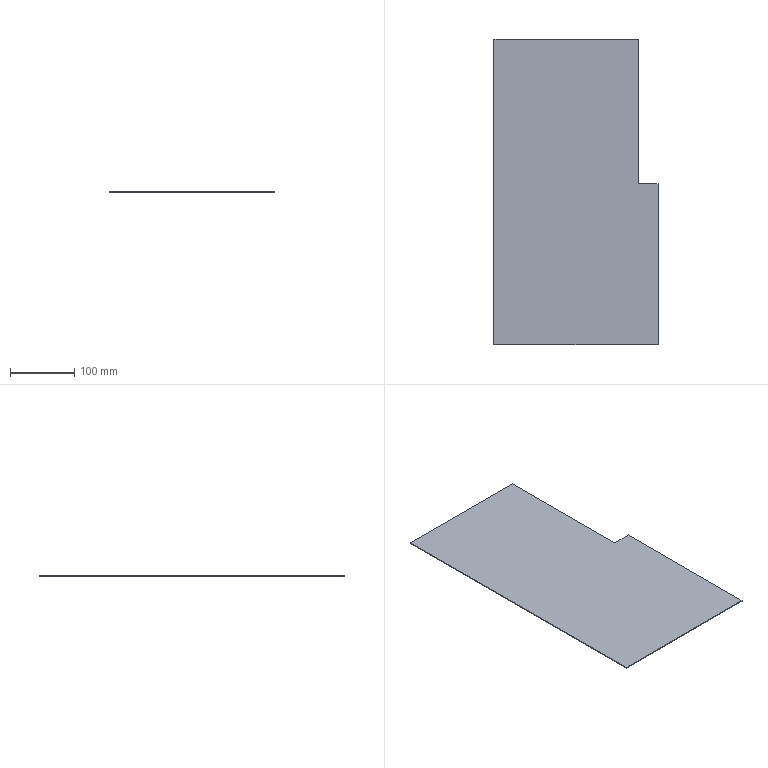Part | 1 solid | 8 faces | box 255 x 475 x 1.2 mm | volume 137250 mm3 | plane 8
STEP:
#1=CARTESIAN_POINT('',(97.5,237.5,0.));
#2=VERTEX_POINT('',#1);
#3=CARTESIAN_POINT('',(97.5,12.5,0.));
#4=VERTEX_POINT('',#3);
#5=CARTESIAN_POINT('',(97.5,0.,0.));
#6=DIRECTION('',(0.,-1.,0.));
#7=VECTOR('',#6,1000.);
#8=LINE('',#5,#7);
#9=EDGE_CURVE('',#2,#4,#8,.T.);
#10=ORIENTED_EDGE('',*,*,#9,.F.);
#11=CARTESIAN_POINT('',(97.5,237.5,1.2));
#12=VERTEX_POINT('',#11);
#13=CARTESIAN_POINT('',(97.5,237.5,1.2));
#14=DIRECTION('',(0.,0.,-1.));
#15=VECTOR('',#14,1000.);
#16=LINE('',#13,#15);
#17=EDGE_CURVE('',#12,#2,#16,.T.);
#18=ORIENTED_EDGE('',*,*,#17,.F.);
#19=CARTESIAN_POINT('',(97.5,12.5,1.2));
#20=VERTEX_POINT('',#19);
#21=CARTESIAN_POINT('',(97.5,0.,1.2));
#22=DIRECTION('',(0.,-1.,0.));
#23=VECTOR('',#22,1000.);
#24=LINE('',#21,#23);
#25=EDGE_CURVE('',#12,#20,#24,.T.);
#26=ORIENTED_EDGE('',*,*,#25,.T.);
#27=CARTESIAN_POINT('',(97.5,12.5,1.2));
#28=DIRECTION('',(0.,0.,-1.));
#29=VECTOR('',#28,1000.);
#30=LINE('',#27,#29);
#31=EDGE_CURVE('',#20,#4,#30,.T.);
#32=ORIENTED_EDGE('',*,*,#31,.T.);
#33=EDGE_LOOP('',(#10,#18,#26,#32));
#34=FACE_OUTER_BOUND('',#33,.T.);
#35=CARTESIAN_POINT('',(97.5,0.,1.2));
#36=DIRECTION('',(1.,0.,0.));
#37=DIRECTION('',(0.,1.,0.));
#38=AXIS2_PLACEMENT_3D('',#35,#36,#37);
#39=PLANE('',#38);
#40=ADVANCED_FACE('',(#34),#39,.T.);
#41=CARTESIAN_POINT('',(-127.5,237.5,0.));
#42=VERTEX_POINT('',#41);
#43=CARTESIAN_POINT('',(0.,237.5,0.));
#44=DIRECTION('',(1.,0.,0.));
#45=VECTOR('',#44,1000.);
#46=LINE('',#43,#45);
#47=EDGE_CURVE('',#42,#2,#46,.T.);
#48=ORIENTED_EDGE('',*,*,#47,.F.);
#49=CARTESIAN_POINT('',(-127.5,237.5,1.2));
#50=VERTEX_POINT('',#49);
#51=CARTESIAN_POINT('',(-127.5,237.5,1.2));
#52=DIRECTION('',(0.,0.,-1.));
#53=VECTOR('',#52,1000.);
#54=LINE('',#51,#53);
#55=EDGE_CURVE('',#50,#42,#54,.T.);
#56=ORIENTED_EDGE('',*,*,#55,.F.);
#57=CARTESIAN_POINT('',(0.,237.5,1.2));
#58=DIRECTION('',(1.,0.,0.));
#59=VECTOR('',#58,1000.);
#60=LINE('',#57,#59);
#61=EDGE_CURVE('',#50,#12,#60,.T.);
#62=ORIENTED_EDGE('',*,*,#61,.T.);
#63=ORIENTED_EDGE('',*,*,#17,.T.);
#64=EDGE_LOOP('',(#48,#56,#62,#63));
#65=FACE_OUTER_BOUND('',#64,.T.);
#66=CARTESIAN_POINT('',(0.,237.5,1.2));
#67=DIRECTION('',(0.,1.,0.));
#68=DIRECTION('',(0.,0.,1.));
#69=AXIS2_PLACEMENT_3D('',#66,#67,#68);
#70=PLANE('',#69);
#71=ADVANCED_FACE('',(#65),#70,.T.);
#72=CARTESIAN_POINT('',(-127.5,-237.5,0.));
#73=VERTEX_POINT('',#72);
#74=CARTESIAN_POINT('',(-127.5,0.,0.));
#75=DIRECTION('',(0.,-1.,0.));
#76=VECTOR('',#75,1000.);
#77=LINE('',#74,#76);
#78=EDGE_CURVE('',#42,#73,#77,.T.);
#79=ORIENTED_EDGE('',*,*,#78,.T.);
#80=CARTESIAN_POINT('',(-127.5,-237.5,1.2));
#81=VERTEX_POINT('',#80);
#82=CARTESIAN_POINT('',(-127.5,-237.5,1.2));
#83=DIRECTION('',(0.,0.,-1.));
#84=VECTOR('',#83,1000.);
#85=LINE('',#82,#84);
#86=EDGE_CURVE('',#81,#73,#85,.T.);
#87=ORIENTED_EDGE('',*,*,#86,.F.);
#88=CARTESIAN_POINT('',(-127.5,0.,1.2));
#89=DIRECTION('',(0.,-1.,0.));
#90=VECTOR('',#89,1000.);
#91=LINE('',#88,#90);
#92=EDGE_CURVE('',#50,#81,#91,.T.);
#93=ORIENTED_EDGE('',*,*,#92,.F.);
#94=ORIENTED_EDGE('',*,*,#55,.T.);
#95=EDGE_LOOP('',(#79,#87,#93,#94));
#96=FACE_OUTER_BOUND('',#95,.T.);
#97=CARTESIAN_POINT('',(-127.5,0.,1.2));
#98=DIRECTION('',(1.,0.,0.));
#99=DIRECTION('',(0.,1.,0.));
#100=AXIS2_PLACEMENT_3D('',#97,#98,#99);
#101=PLANE('',#100);
#102=ADVANCED_FACE('',(#96),#101,.F.);
#103=CARTESIAN_POINT('',(127.5,-237.5,0.));
#104=VERTEX_POINT('',#103);
#105=CARTESIAN_POINT('',(0.,-237.5,0.));
#106=DIRECTION('',(1.,0.,0.));
#107=VECTOR('',#106,1000.);
#108=LINE('',#105,#107);
#109=EDGE_CURVE('',#73,#104,#108,.T.);
#110=ORIENTED_EDGE('',*,*,#109,.T.);
#111=CARTESIAN_POINT('',(127.5,-237.5,1.2));
#112=VERTEX_POINT('',#111);
#113=CARTESIAN_POINT('',(127.5,-237.5,1.2));
#114=DIRECTION('',(0.,0.,-1.));
#115=VECTOR('',#114,1000.);
#116=LINE('',#113,#115);
#117=EDGE_CURVE('',#112,#104,#116,.T.);
#118=ORIENTED_EDGE('',*,*,#117,.F.);
#119=CARTESIAN_POINT('',(0.,-237.5,1.2));
#120=DIRECTION('',(1.,0.,0.));
#121=VECTOR('',#120,1000.);
#122=LINE('',#119,#121);
#123=EDGE_CURVE('',#81,#112,#122,.T.);
#124=ORIENTED_EDGE('',*,*,#123,.F.);
#125=ORIENTED_EDGE('',*,*,#86,.T.);
#126=EDGE_LOOP('',(#110,#118,#124,#125));
#127=FACE_OUTER_BOUND('',#126,.T.);
#128=CARTESIAN_POINT('',(0.,-237.5,1.2));
#129=DIRECTION('',(0.,1.,0.));
#130=DIRECTION('',(0.,0.,1.));
#131=AXIS2_PLACEMENT_3D('',#128,#129,#130);
#132=PLANE('',#131);
#133=ADVANCED_FACE('',(#127),#132,.F.);
#134=CARTESIAN_POINT('',(127.5,12.5,0.));
#135=VERTEX_POINT('',#134);
#136=CARTESIAN_POINT('',(127.5,0.,0.));
#137=DIRECTION('',(0.,-1.,0.));
#138=VECTOR('',#137,1000.);
#139=LINE('',#136,#138);
#140=EDGE_CURVE('',#135,#104,#139,.T.);
#141=ORIENTED_EDGE('',*,*,#140,.F.);
#142=CARTESIAN_POINT('',(127.5,12.5,1.2));
#143=VERTEX_POINT('',#142);
#144=CARTESIAN_POINT('',(127.5,12.5,1.2));
#145=DIRECTION('',(0.,0.,-1.));
#146=VECTOR('',#145,1000.);
#147=LINE('',#144,#146);
#148=EDGE_CURVE('',#143,#135,#147,.T.);
#149=ORIENTED_EDGE('',*,*,#148,.F.);
#150=CARTESIAN_POINT('',(127.5,0.,1.2));
#151=DIRECTION('',(0.,-1.,0.));
#152=VECTOR('',#151,1000.);
#153=LINE('',#150,#152);
#154=EDGE_CURVE('',#143,#112,#153,.T.);
#155=ORIENTED_EDGE('',*,*,#154,.T.);
#156=ORIENTED_EDGE('',*,*,#117,.T.);
#157=EDGE_LOOP('',(#141,#149,#155,#156));
#158=FACE_OUTER_BOUND('',#157,.T.);
#159=CARTESIAN_POINT('',(127.5,0.,1.2));
#160=DIRECTION('',(1.,0.,0.));
#161=DIRECTION('',(0.,1.,0.));
#162=AXIS2_PLACEMENT_3D('',#159,#160,#161);
#163=PLANE('',#162);
#164=ADVANCED_FACE('',(#158),#163,.T.);
#165=CARTESIAN_POINT('',(0.,12.5,0.));
#166=DIRECTION('',(-1.,0.,0.));
#167=VECTOR('',#166,1000.);
#168=LINE('',#165,#167);
#169=EDGE_CURVE('',#135,#4,#168,.T.);
#170=ORIENTED_EDGE('',*,*,#169,.T.);
#171=ORIENTED_EDGE('',*,*,#31,.F.);
#172=CARTESIAN_POINT('',(0.,12.5,1.2));
#173=DIRECTION('',(-1.,0.,0.));
#174=VECTOR('',#173,1000.);
#175=LINE('',#172,#174);
#176=EDGE_CURVE('',#143,#20,#175,.T.);
#177=ORIENTED_EDGE('',*,*,#176,.F.);
#178=ORIENTED_EDGE('',*,*,#148,.T.);
#179=EDGE_LOOP('',(#170,#171,#177,#178));
#180=FACE_OUTER_BOUND('',#179,.T.);
#181=CARTESIAN_POINT('',(0.,12.5,1.2));
#182=DIRECTION('',(0.,-1.,0.));
#183=DIRECTION('',(1.,0.,0.));
#184=AXIS2_PLACEMENT_3D('',#181,#182,#183);
#185=PLANE('',#184);
#186=ADVANCED_FACE('',(#180),#185,.F.);
#187=ORIENTED_EDGE('',*,*,#25,.F.);
#188=ORIENTED_EDGE('',*,*,#61,.F.);
#189=ORIENTED_EDGE('',*,*,#92,.T.);
#190=ORIENTED_EDGE('',*,*,#123,.T.);
#191=ORIENTED_EDGE('',*,*,#154,.F.);
#192=ORIENTED_EDGE('',*,*,#176,.T.);
#193=EDGE_LOOP('',(#187,#188,#189,#190,#191,#192));
#194=FACE_OUTER_BOUND('',#193,.T.);
#195=CARTESIAN_POINT('',(0.,0.,1.2));
#196=DIRECTION('',(0.,0.,1.));
#197=DIRECTION('',(1.,0.,0.));
#198=AXIS2_PLACEMENT_3D('',#195,#196,#197);
#199=PLANE('',#198);
#200=ADVANCED_FACE('',(#194),#199,.T.);
#201=ORIENTED_EDGE('',*,*,#9,.T.);
#202=ORIENTED_EDGE('',*,*,#169,.F.);
#203=ORIENTED_EDGE('',*,*,#140,.T.);
#204=ORIENTED_EDGE('',*,*,#109,.F.);
#205=ORIENTED_EDGE('',*,*,#78,.F.);
#206=ORIENTED_EDGE('',*,*,#47,.T.);
#207=EDGE_LOOP('',(#201,#202,#203,#204,#205,#206));
#208=FACE_OUTER_BOUND('',#207,.T.);
#209=CARTESIAN_POINT('',(0.,0.,0.));
#210=DIRECTION('',(0.,0.,1.));
#211=DIRECTION('',(1.,0.,0.));
#212=AXIS2_PLACEMENT_3D('',#209,#210,#211);
#213=PLANE('',#212);
#214=ADVANCED_FACE('',(#208),#213,.F.);
#215=CLOSED_SHELL('',(#40,#71,#102,#133,#164,#186,#200,#214));
#216=MANIFOLD_SOLID_BREP('',#215);
#217=CARTESIAN_POINT('',(0.,0.,0.));
#218=DIRECTION('',(0.,0.,1.));
#219=DIRECTION('',(1.,0.,0.));
#220=AXIS2_PLACEMENT_3D('',#217,#218,#219);
#221=(LENGTH_UNIT()NAMED_UNIT(*)SI_UNIT(.MILLI.,.METRE.));
#222=UNCERTAINTY_MEASURE_WITH_UNIT(LENGTH_MEASURE(0.00001),#221,'','');
#223=(NAMED_UNIT(*)PLANE_ANGLE_UNIT()SI_UNIT($,.RADIAN.));
#224=(NAMED_UNIT(*)SI_UNIT($,.STERADIAN.)SOLID_ANGLE_UNIT());
#225=(GEOMETRIC_REPRESENTATION_CONTEXT(3)GLOBAL_UNCERTAINTY_ASSIGNED_CONTEXT((#222))GLOBAL_UNIT_ASSIGNED_CONTEXT((#221,#223,#224))REPRESENTATION_CONTEXT('',''));
#226=ADVANCED_BREP_SHAPE_REPRESENTATION('',(#216,#220),#225);